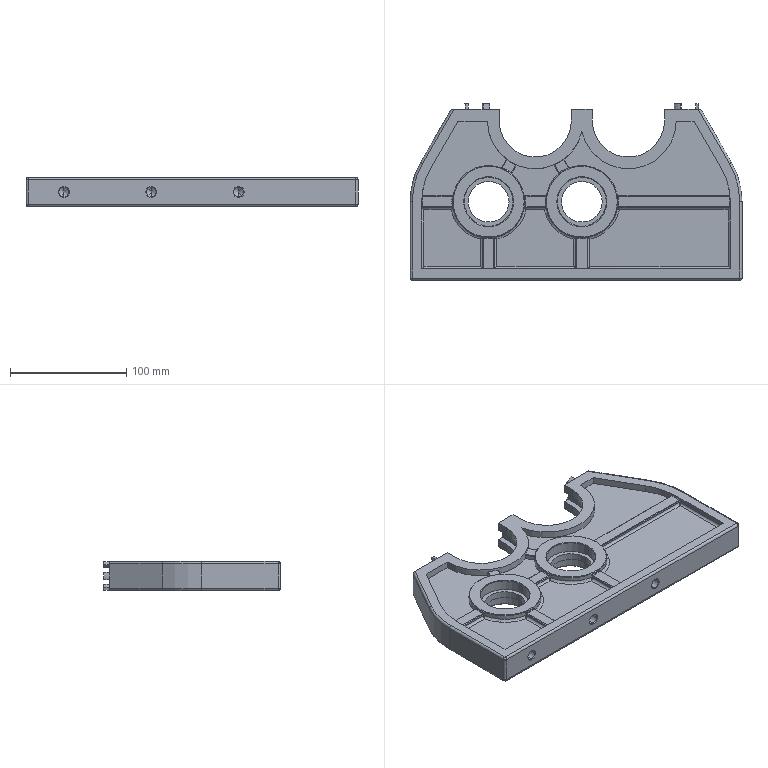Part | SolidWorks | features ICE 5, MoveFace 2, BaseBody 1, CombineBodies 1, DeleteBody 1, ExtruRefSurface 1, MirrorSolid 1, Split 1 | 1 solid | 440 faces | box 285 x 151.742 x 25 mm | volume 571521 mm3 | plane 216 | cylinder 92 | spline 64 | cone 52 | torus 12 | sphere 4 | commonest cylinder face diameters 4 x36 62 x12 42 x8 8.5 x6 20 x6 25 x6